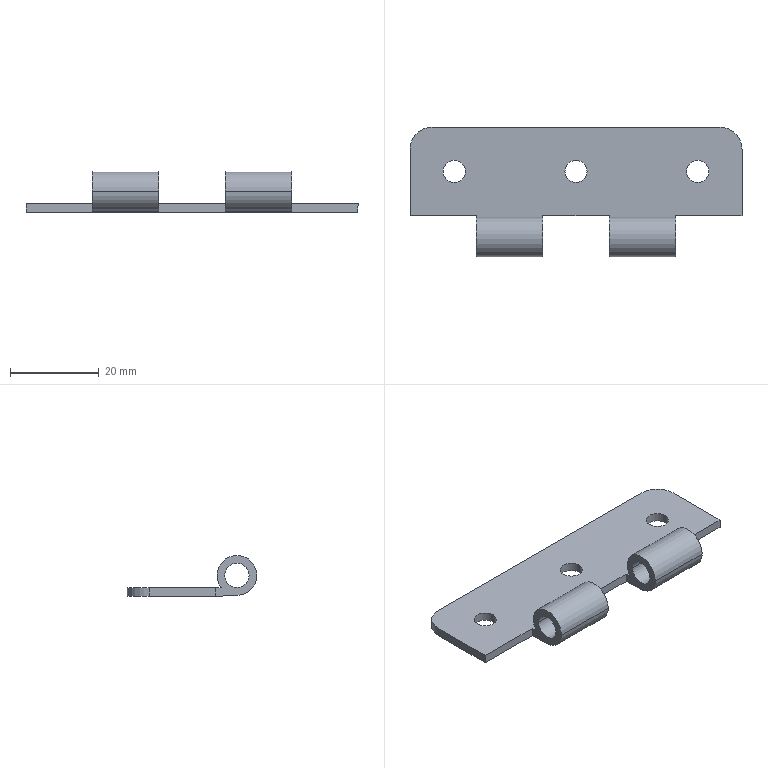Part | SolidWorks | features Extrusion 1, Fillet 1, ICE 1, LPattern 1 | 1 solid | 32 faces | box 75 x 29.3 x 9.25 mm | volume 4196 mm3 | cylinder 18 | plane 14 | commonest cylinder face diameters 5 x6 9 x6 5.5 x4 10 x2
STEP:
#1=CARTESIAN_POINT('',(60.,-22.05,4.75));
#2=VERTEX_POINT('',#1);
#3=CARTESIAN_POINT('',(60.,-27.55,4.75));
#4=VERTEX_POINT('',#3);
#5=CARTESIAN_POINT('',(60.,-24.8,4.75));
#6=DIRECTION('',(-1.,0.,0.));
#7=DIRECTION('',(0.,-1.,0.));
#8=AXIS2_PLACEMENT_3D('',#5,#6,#7);
#9=CIRCLE('',#8,2.75);
#10=EDGE_CURVE('',#2,#4,#9,.T.);
#11=ORIENTED_EDGE('',*,*,#10,.F.);
#12=CARTESIAN_POINT('',(45.,-22.05,4.75));
#13=VERTEX_POINT('',#12);
#14=CARTESIAN_POINT('',(60.,-22.05,4.75));
#15=DIRECTION('',(-1.,0.,0.));
#16=VECTOR('',#15,1000.);
#17=LINE('',#14,#16);
#18=EDGE_CURVE('',#2,#13,#17,.T.);
#19=ORIENTED_EDGE('',*,*,#18,.T.);
#20=CARTESIAN_POINT('',(45.,-27.55,4.75));
#21=VERTEX_POINT('',#20);
#22=CARTESIAN_POINT('',(45.,-24.8,4.75));
#23=DIRECTION('',(-1.,0.,0.));
#24=DIRECTION('',(0.,-1.,0.));
#25=AXIS2_PLACEMENT_3D('',#22,#23,#24);
#26=CIRCLE('',#25,2.75);
#27=EDGE_CURVE('',#13,#21,#26,.T.);
#28=ORIENTED_EDGE('',*,*,#27,.T.);
#29=CARTESIAN_POINT('',(60.,-27.55,4.75));
#30=DIRECTION('',(-1.,0.,0.));
#31=VECTOR('',#30,1000.);
#32=LINE('',#29,#31);
#33=EDGE_CURVE('',#4,#21,#32,.T.);
#34=ORIENTED_EDGE('',*,*,#33,.F.);
#35=EDGE_LOOP('',(#11,#19,#28,#34));
#36=FACE_OUTER_BOUND('',#35,.T.);
#37=CARTESIAN_POINT('',(60.,-24.8,4.75));
#38=DIRECTION('',(-1.,0.,0.));
#39=DIRECTION('',(0.,-1.,0.));
#40=AXIS2_PLACEMENT_3D('',#37,#38,#39);
#41=CYLINDRICAL_SURFACE('',#40,2.75);
#42=ADVANCED_FACE('',(#36),#41,.F.);
#43=CARTESIAN_POINT('',(60.,-29.3,4.75));
#44=VERTEX_POINT('',#43);
#45=CARTESIAN_POINT('',(60.,-20.3,4.75));
#46=VERTEX_POINT('',#45);
#47=CARTESIAN_POINT('',(60.,-24.8,4.75));
#48=DIRECTION('',(-1.,0.,0.));
#49=DIRECTION('',(0.,-1.,0.));
#50=AXIS2_PLACEMENT_3D('',#47,#48,#49);
#51=CIRCLE('',#50,4.5);
#52=EDGE_CURVE('',#44,#46,#51,.T.);
#53=ORIENTED_EDGE('',*,*,#52,.T.);
#54=CARTESIAN_POINT('',(45.,-20.3,4.75));
#55=VERTEX_POINT('',#54);
#56=CARTESIAN_POINT('',(60.,-20.3,4.75));
#57=DIRECTION('',(-1.,0.,0.));
#58=VECTOR('',#57,1000.);
#59=LINE('',#56,#58);
#60=EDGE_CURVE('',#46,#55,#59,.T.);
#61=ORIENTED_EDGE('',*,*,#60,.T.);
#62=CARTESIAN_POINT('',(45.,-29.3,4.75));
#63=VERTEX_POINT('',#62);
#64=CARTESIAN_POINT('',(45.,-24.8,4.75));
#65=DIRECTION('',(-1.,0.,0.));
#66=DIRECTION('',(0.,-1.,0.));
#67=AXIS2_PLACEMENT_3D('',#64,#65,#66);
#68=CIRCLE('',#67,4.5);
#69=EDGE_CURVE('',#63,#55,#68,.T.);
#70=ORIENTED_EDGE('',*,*,#69,.F.);
#71=CARTESIAN_POINT('',(60.,-29.3,4.75));
#72=DIRECTION('',(-1.,0.,0.));
#73=VECTOR('',#72,1000.);
#74=LINE('',#71,#73);
#75=EDGE_CURVE('',#44,#63,#74,.T.);
#76=ORIENTED_EDGE('',*,*,#75,.F.);
#77=EDGE_LOOP('',(#53,#61,#70,#76));
#78=FACE_OUTER_BOUND('',#77,.T.);
#79=CARTESIAN_POINT('',(60.,-24.8,4.75));
#80=DIRECTION('',(-1.,0.,0.));
#81=DIRECTION('',(0.,-1.,0.));
#82=AXIS2_PLACEMENT_3D('',#79,#80,#81);
#83=CYLINDRICAL_SURFACE('',#82,4.5);
#84=ADVANCED_FACE('',(#78),#83,.T.);
#85=CARTESIAN_POINT('',(60.,-25.029,0.2558));
#86=VERTEX_POINT('',#85);
#87=CARTESIAN_POINT('',(60.,-24.8,4.75));
#88=DIRECTION('',(-1.,0.,0.));
#89=DIRECTION('',(0.,-1.,0.));
#90=AXIS2_PLACEMENT_3D('',#87,#88,#89);
#91=CIRCLE('',#90,4.5);
#92=EDGE_CURVE('',#86,#44,#91,.T.);
#93=ORIENTED_EDGE('',*,*,#92,.T.);
#94=ORIENTED_EDGE('',*,*,#75,.T.);
#95=CARTESIAN_POINT('',(45.,-25.029,0.2558));
#96=VERTEX_POINT('',#95);
#97=CARTESIAN_POINT('',(45.,-24.8,4.75));
#98=DIRECTION('',(-1.,0.,0.));
#99=DIRECTION('',(0.,-1.,0.));
#100=AXIS2_PLACEMENT_3D('',#97,#98,#99);
#101=CIRCLE('',#100,4.5);
#102=EDGE_CURVE('',#96,#63,#101,.T.);
#103=ORIENTED_EDGE('',*,*,#102,.F.);
#104=CARTESIAN_POINT('',(60.,-25.029,0.2558));
#105=DIRECTION('',(-1.,0.,0.));
#106=VECTOR('',#105,1000.);
#107=LINE('',#104,#106);
#108=EDGE_CURVE('',#86,#96,#107,.T.);
#109=ORIENTED_EDGE('',*,*,#108,.F.);
#110=EDGE_LOOP('',(#93,#94,#103,#109));
#111=FACE_OUTER_BOUND('',#110,.T.);
#112=CARTESIAN_POINT('',(60.,-24.8,4.75));
#113=DIRECTION('',(-1.,0.,0.));
#114=DIRECTION('',(0.,-1.,0.));
#115=AXIS2_PLACEMENT_3D('',#112,#113,#114);
#116=CYLINDRICAL_SURFACE('',#115,4.5);
#117=ADVANCED_FACE('',(#111),#116,.T.);
#118=CARTESIAN_POINT('',(30.,-22.05,4.75));
#119=VERTEX_POINT('',#118);
#120=CARTESIAN_POINT('',(30.,-27.55,4.75));
#121=VERTEX_POINT('',#120);
#122=CARTESIAN_POINT('',(30.,-24.8,4.75));
#123=DIRECTION('',(-1.,0.,0.));
#124=DIRECTION('',(0.,-1.,0.));
#125=AXIS2_PLACEMENT_3D('',#122,#123,#124);
#126=CIRCLE('',#125,2.75);
#127=EDGE_CURVE('',#119,#121,#126,.T.);
#128=ORIENTED_EDGE('',*,*,#127,.F.);
#129=CARTESIAN_POINT('',(15.,-22.05,4.75));
#130=VERTEX_POINT('',#129);
#131=CARTESIAN_POINT('',(30.,-22.05,4.75));
#132=DIRECTION('',(-1.,0.,0.));
#133=VECTOR('',#132,1000.);
#134=LINE('',#131,#133);
#135=EDGE_CURVE('',#119,#130,#134,.T.);
#136=ORIENTED_EDGE('',*,*,#135,.T.);
#137=CARTESIAN_POINT('',(15.,-27.55,4.75));
#138=VERTEX_POINT('',#137);
#139=CARTESIAN_POINT('',(15.,-24.8,4.75));
#140=DIRECTION('',(-1.,0.,0.));
#141=DIRECTION('',(0.,-1.,0.));
#142=AXIS2_PLACEMENT_3D('',#139,#140,#141);
#143=CIRCLE('',#142,2.75);
#144=EDGE_CURVE('',#130,#138,#143,.T.);
#145=ORIENTED_EDGE('',*,*,#144,.T.);
#146=CARTESIAN_POINT('',(30.,-27.55,4.75));
#147=DIRECTION('',(-1.,0.,0.));
#148=VECTOR('',#147,1000.);
#149=LINE('',#146,#148);
#150=EDGE_CURVE('',#121,#138,#149,.T.);
#151=ORIENTED_EDGE('',*,*,#150,.F.);
#152=EDGE_LOOP('',(#128,#136,#145,#151));
#153=FACE_OUTER_BOUND('',#152,.T.);
#154=CARTESIAN_POINT('',(30.,-24.8,4.75));
#155=DIRECTION('',(-1.,0.,0.));
#156=DIRECTION('',(0.,-1.,0.));
#157=AXIS2_PLACEMENT_3D('',#154,#155,#156);
#158=CYLINDRICAL_SURFACE('',#157,2.75);
#159=ADVANCED_FACE('',(#153),#158,.F.);
#160=CARTESIAN_POINT('',(30.,-29.3,4.75));
#161=VERTEX_POINT('',#160);
#162=CARTESIAN_POINT('',(30.,-20.3,4.75));
#163=VERTEX_POINT('',#162);
#164=CARTESIAN_POINT('',(30.,-24.8,4.75));
#165=DIRECTION('',(-1.,0.,0.));
#166=DIRECTION('',(0.,-1.,0.));
#167=AXIS2_PLACEMENT_3D('',#164,#165,#166);
#168=CIRCLE('',#167,4.5);
#169=EDGE_CURVE('',#161,#163,#168,.T.);
#170=ORIENTED_EDGE('',*,*,#169,.T.);
#171=CARTESIAN_POINT('',(15.,-20.3,4.75));
#172=VERTEX_POINT('',#171);
#173=CARTESIAN_POINT('',(30.,-20.3,4.75));
#174=DIRECTION('',(-1.,0.,0.));
#175=VECTOR('',#174,1000.);
#176=LINE('',#173,#175);
#177=EDGE_CURVE('',#163,#172,#176,.T.);
#178=ORIENTED_EDGE('',*,*,#177,.T.);
#179=CARTESIAN_POINT('',(15.,-29.3,4.75));
#180=VERTEX_POINT('',#179);
#181=CARTESIAN_POINT('',(15.,-24.8,4.75));
#182=DIRECTION('',(-1.,0.,0.));
#183=DIRECTION('',(0.,-1.,0.));
#184=AXIS2_PLACEMENT_3D('',#181,#182,#183);
#185=CIRCLE('',#184,4.5);
#186=EDGE_CURVE('',#180,#172,#185,.T.);
#187=ORIENTED_EDGE('',*,*,#186,.F.);
#188=CARTESIAN_POINT('',(30.,-29.3,4.75));
#189=DIRECTION('',(-1.,0.,0.));
#190=VECTOR('',#189,1000.);
#191=LINE('',#188,#190);
#192=EDGE_CURVE('',#161,#180,#191,.T.);
#193=ORIENTED_EDGE('',*,*,#192,.F.);
#194=EDGE_LOOP('',(#170,#178,#187,#193));
#195=FACE_OUTER_BOUND('',#194,.T.);
#196=CARTESIAN_POINT('',(30.,-24.8,4.75));
#197=DIRECTION('',(-1.,0.,0.));
#198=DIRECTION('',(0.,-1.,0.));
#199=AXIS2_PLACEMENT_3D('',#196,#197,#198);
#200=CYLINDRICAL_SURFACE('',#199,4.5);
#201=ADVANCED_FACE('',(#195),#200,.T.);
#202=CARTESIAN_POINT('',(30.,-25.029,0.2558));
#203=VERTEX_POINT('',#202);
#204=CARTESIAN_POINT('',(30.,-24.8,4.75));
#205=DIRECTION('',(-1.,0.,0.));
#206=DIRECTION('',(0.,-1.,0.));
#207=AXIS2_PLACEMENT_3D('',#204,#205,#206);
#208=CIRCLE('',#207,4.5);
#209=EDGE_CURVE('',#203,#161,#208,.T.);
#210=ORIENTED_EDGE('',*,*,#209,.T.);
#211=ORIENTED_EDGE('',*,*,#192,.T.);
#212=CARTESIAN_POINT('',(15.,-25.029,0.2558));
#213=VERTEX_POINT('',#212);
#214=CARTESIAN_POINT('',(15.,-24.8,4.75));
#215=DIRECTION('',(-1.,0.,0.));
#216=DIRECTION('',(0.,-1.,0.));
#217=AXIS2_PLACEMENT_3D('',#214,#215,#216);
#218=CIRCLE('',#217,4.5);
#219=EDGE_CURVE('',#213,#180,#218,.T.);
#220=ORIENTED_EDGE('',*,*,#219,.F.);
#221=CARTESIAN_POINT('',(30.,-25.029,0.2558));
#222=DIRECTION('',(-1.,0.,0.));
#223=VECTOR('',#222,1000.);
#224=LINE('',#221,#223);
#225=EDGE_CURVE('',#203,#213,#224,.T.);
#226=ORIENTED_EDGE('',*,*,#225,.F.);
#227=EDGE_LOOP('',(#210,#211,#220,#226));
#228=FACE_OUTER_BOUND('',#227,.T.);
#229=CARTESIAN_POINT('',(30.,-24.8,4.75));
#230=DIRECTION('',(-1.,0.,0.));
#231=DIRECTION('',(0.,-1.,0.));
#232=AXIS2_PLACEMENT_3D('',#229,#230,#231);
#233=CYLINDRICAL_SURFACE('',#232,4.5);
#234=ADVANCED_FACE('',(#228),#233,.T.);
#235=CARTESIAN_POINT('',(35.,-10.,2.));
#236=VERTEX_POINT('',#235);
#237=CARTESIAN_POINT('',(40.,-10.,2.));
#238=VERTEX_POINT('',#237);
#239=CARTESIAN_POINT('',(37.5,-10.,2.));
#240=DIRECTION('',(0.,0.,1.));
#241=DIRECTION('',(1.,0.,0.));
#242=AXIS2_PLACEMENT_3D('',#239,#240,#241);
#243=CIRCLE('',#242,2.5);
#244=EDGE_CURVE('',#236,#238,#243,.T.);
#245=ORIENTED_EDGE('',*,*,#244,.T.);
#246=CARTESIAN_POINT('',(40.,-10.,0.));
#247=VERTEX_POINT('',#246);
#248=CARTESIAN_POINT('',(40.,-10.,2.));
#249=DIRECTION('',(0.,0.,-1.));
#250=VECTOR('',#249,1000.);
#251=LINE('',#248,#250);
#252=EDGE_CURVE('',#238,#247,#251,.T.);
#253=ORIENTED_EDGE('',*,*,#252,.T.);
#254=CARTESIAN_POINT('',(35.,-10.,0.));
#255=VERTEX_POINT('',#254);
#256=CARTESIAN_POINT('',(37.5,-10.,0.));
#257=DIRECTION('',(0.,0.,1.));
#258=DIRECTION('',(1.,0.,0.));
#259=AXIS2_PLACEMENT_3D('',#256,#257,#258);
#260=CIRCLE('',#259,2.5);
#261=EDGE_CURVE('',#255,#247,#260,.T.);
#262=ORIENTED_EDGE('',*,*,#261,.F.);
#263=CARTESIAN_POINT('',(35.,-10.,2.));
#264=DIRECTION('',(0.,0.,-1.));
#265=VECTOR('',#264,1000.);
#266=LINE('',#263,#265);
#267=EDGE_CURVE('',#236,#255,#266,.T.);
#268=ORIENTED_EDGE('',*,*,#267,.F.);
#269=EDGE_LOOP('',(#245,#253,#262,#268));
#270=FACE_OUTER_BOUND('',#269,.T.);
#271=CARTESIAN_POINT('',(37.5,-10.,2.));
#272=DIRECTION('',(0.,0.,-1.));
#273=DIRECTION('',(-1.,0.,0.));
#274=AXIS2_PLACEMENT_3D('',#271,#272,#273);
#275=CYLINDRICAL_SURFACE('',#274,2.5);
#276=ADVANCED_FACE('',(#270),#275,.F.);
#277=CARTESIAN_POINT('',(62.5,-10.,2.));
#278=VERTEX_POINT('',#277);
#279=CARTESIAN_POINT('',(67.5,-10.,2.));
#280=VERTEX_POINT('',#279);
#281=CARTESIAN_POINT('',(65.,-10.,2.));
#282=DIRECTION('',(0.,0.,1.));
#283=DIRECTION('',(1.,0.,0.));
#284=AXIS2_PLACEMENT_3D('',#281,#282,#283);
#285=CIRCLE('',#284,2.5);
#286=EDGE_CURVE('',#278,#280,#285,.T.);
#287=ORIENTED_EDGE('',*,*,#286,.T.);
#288=CARTESIAN_POINT('',(67.5,-10.,0.));
#289=VERTEX_POINT('',#288);
#290=CARTESIAN_POINT('',(67.5,-10.,2.));
#291=DIRECTION('',(0.,0.,-1.));
#292=VECTOR('',#291,1000.);
#293=LINE('',#290,#292);
#294=EDGE_CURVE('',#280,#289,#293,.T.);
#295=ORIENTED_EDGE('',*,*,#294,.T.);
#296=CARTESIAN_POINT('',(62.5,-10.,0.));
#297=VERTEX_POINT('',#296);
#298=CARTESIAN_POINT('',(65.,-10.,0.));
#299=DIRECTION('',(0.,0.,1.));
#300=DIRECTION('',(1.,0.,0.));
#301=AXIS2_PLACEMENT_3D('',#298,#299,#300);
#302=CIRCLE('',#301,2.5);
#303=EDGE_CURVE('',#297,#289,#302,.T.);
#304=ORIENTED_EDGE('',*,*,#303,.F.);
#305=CARTESIAN_POINT('',(62.5,-10.,2.));
#306=DIRECTION('',(0.,0.,-1.));
#307=VECTOR('',#306,1000.);
#308=LINE('',#305,#307);
#309=EDGE_CURVE('',#278,#297,#308,.T.);
#310=ORIENTED_EDGE('',*,*,#309,.F.);
#311=EDGE_LOOP('',(#287,#295,#304,#310));
#312=FACE_OUTER_BOUND('',#311,.T.);
#313=CARTESIAN_POINT('',(65.,-10.,2.));
#314=DIRECTION('',(0.,0.,-1.));
#315=DIRECTION('',(-1.,0.,0.));
#316=AXIS2_PLACEMENT_3D('',#313,#314,#315);
#317=CYLINDRICAL_SURFACE('',#316,2.5);
#318=ADVANCED_FACE('',(#312),#317,.F.);
#319=CARTESIAN_POINT('',(7.5,-10.,2.));
#320=VERTEX_POINT('',#319);
#321=CARTESIAN_POINT('',(12.5,-10.,2.));
#322=VERTEX_POINT('',#321);
#323=CARTESIAN_POINT('',(10.,-10.,2.));
#324=DIRECTION('',(0.,0.,1.));
#325=DIRECTION('',(1.,0.,0.));
#326=AXIS2_PLACEMENT_3D('',#323,#324,#325);
#327=CIRCLE('',#326,2.5);
#328=EDGE_CURVE('',#320,#322,#327,.T.);
#329=ORIENTED_EDGE('',*,*,#328,.T.);
#330=CARTESIAN_POINT('',(12.5,-10.,0.));
#331=VERTEX_POINT('',#330);
#332=CARTESIAN_POINT('',(12.5,-10.,2.));
#333=DIRECTION('',(0.,0.,-1.));
#334=VECTOR('',#333,1000.);
#335=LINE('',#332,#334);
#336=EDGE_CURVE('',#322,#331,#335,.T.);
#337=ORIENTED_EDGE('',*,*,#336,.T.);
#338=CARTESIAN_POINT('',(7.5,-10.,0.));
#339=VERTEX_POINT('',#338);
#340=CARTESIAN_POINT('',(10.,-10.,0.));
#341=DIRECTION('',(0.,0.,1.));
#342=DIRECTION('',(1.,0.,0.));
#343=AXIS2_PLACEMENT_3D('',#340,#341,#342);
#344=CIRCLE('',#343,2.5);
#345=EDGE_CURVE('',#339,#331,#344,.T.);
#346=ORIENTED_EDGE('',*,*,#345,.F.);
#347=CARTESIAN_POINT('',(7.5,-10.,2.));
#348=DIRECTION('',(0.,0.,-1.));
#349=VECTOR('',#348,1000.);
#350=LINE('',#347,#349);
#351=EDGE_CURVE('',#320,#339,#350,.T.);
#352=ORIENTED_EDGE('',*,*,#351,.F.);
#353=EDGE_LOOP('',(#329,#337,#346,#352));
#354=FACE_OUTER_BOUND('',#353,.T.);
#355=CARTESIAN_POINT('',(10.,-10.,2.));
#356=DIRECTION('',(0.,0.,-1.));
#357=DIRECTION('',(-1.,0.,0.));
#358=AXIS2_PLACEMENT_3D('',#355,#356,#357);
#359=CYLINDRICAL_SURFACE('',#358,2.5);
#360=ADVANCED_FACE('',(#354),#359,.F.);
#361=CARTESIAN_POINT('',(60.,-20.,0.));
#362=VERTEX_POINT('',#361);
#363=CARTESIAN_POINT('',(60.,-20.,2.));
#364=VERTEX_POINT('',#363);
#365=CARTESIAN_POINT('',(60.,-20.,0.));
#366=DIRECTION('',(0.,0.,1.));
#367=VECTOR('',#366,1000.);
#368=LINE('',#365,#367);
#369=EDGE_CURVE('',#362,#364,#368,.T.);
#370=ORIENTED_EDGE('',*,*,#369,.F.);
#371=CARTESIAN_POINT('',(75.,-20.,0.));
#372=VERTEX_POINT('',#371);
#373=CARTESIAN_POINT('',(0.,-20.,0.));
#374=DIRECTION('',(1.,0.,0.));
#375=VECTOR('',#374,1000.);
#376=LINE('',#373,#375);
#377=EDGE_CURVE('',#362,#372,#376,.T.);
#378=ORIENTED_EDGE('',*,*,#377,.T.);
#379=CARTESIAN_POINT('',(75.,-20.,2.));
#380=VERTEX_POINT('',#379);
#381=CARTESIAN_POINT('',(75.,-20.,2.));
#382=DIRECTION('',(0.,0.,-1.));
#383=VECTOR('',#382,1000.);
#384=LINE('',#381,#383);
#385=EDGE_CURVE('',#380,#372,#384,.T.);
#386=ORIENTED_EDGE('',*,*,#385,.F.);
#387=CARTESIAN_POINT('',(0.,-20.,2.));
#388=DIRECTION('',(1.,0.,0.));
#389=VECTOR('',#388,1000.);
#390=LINE('',#387,#389);
#391=EDGE_CURVE('',#364,#380,#390,.T.);
#392=ORIENTED_EDGE('',*,*,#391,.F.);
#393=EDGE_LOOP('',(#370,#378,#386,#392));
#394=FACE_OUTER_BOUND('',#393,.T.);
#395=CARTESIAN_POINT('',(0.,-20.,2.));
#396=DIRECTION('',(0.,1.,0.));
#397=DIRECTION('',(0.,0.,1.));
#398=AXIS2_PLACEMENT_3D('',#395,#396,#397);
#399=PLANE('',#398);
#400=ADVANCED_FACE('',(#394),#399,.F.);
#401=CARTESIAN_POINT('',(30.,-20.,0.));
#402=VERTEX_POINT('',#401);
#403=CARTESIAN_POINT('',(45.,-20.,0.));
#404=VERTEX_POINT('',#403);
#405=CARTESIAN_POINT('',(0.,-20.,0.));
#406=DIRECTION('',(1.,0.,0.));
#407=VECTOR('',#406,1000.);
#408=LINE('',#405,#407);
#409=EDGE_CURVE('',#402,#404,#408,.T.);
#410=ORIENTED_EDGE('',*,*,#409,.T.);
#411=CARTESIAN_POINT('',(45.,-20.,2.));
#412=VERTEX_POINT('',#411);
#413=CARTESIAN_POINT('',(45.,-20.,0.));
#414=DIRECTION('',(0.,0.,1.));
#415=VECTOR('',#414,1000.);
#416=LINE('',#413,#415);
#417=EDGE_CURVE('',#404,#412,#416,.T.);
#418=ORIENTED_EDGE('',*,*,#417,.T.);
#419=CARTESIAN_POINT('',(30.,-20.,2.));
#420=VERTEX_POINT('',#419);
#421=CARTESIAN_POINT('',(0.,-20.,2.));
#422=DIRECTION('',(1.,0.,0.));
#423=VECTOR('',#422,1000.);
#424=LINE('',#421,#423);
#425=EDGE_CURVE('',#420,#412,#424,.T.);
#426=ORIENTED_EDGE('',*,*,#425,.F.);
#427=CARTESIAN_POINT('',(30.,-20.,0.));
#428=DIRECTION('',(0.,0.,1.));
#429=VECTOR('',#428,1000.);
#430=LINE('',#427,#429);
#431=EDGE_CURVE('',#402,#420,#430,.T.);
#432=ORIENTED_EDGE('',*,*,#431,.F.);
#433=EDGE_LOOP('',(#410,#418,#426,#432));
#434=FACE_OUTER_BOUND('',#433,.T.);
#435=CARTESIAN_POINT('',(0.,-20.,2.));
#436=DIRECTION('',(0.,1.,0.));
#437=DIRECTION('',(0.,0.,1.));
#438=AXIS2_PLACEMENT_3D('',#435,#436,#437);
#439=PLANE('',#438);
#440=ADVANCED_FACE('',(#434),#439,.F.);
#441=ORIENTED_EDGE('',*,*,#286,.F.);
#442=CARTESIAN_POINT('',(65.,-10.,2.));
#443=DIRECTION('',(0.,0.,1.));
#444=DIRECTION('',(1.,0.,0.));
#445=AXIS2_PLACEMENT_3D('',#442,#443,#444);
#446=CIRCLE('',#445,2.5);
#447=EDGE_CURVE('',#280,#278,#446,.T.);
#448=ORIENTED_EDGE('',*,*,#447,.F.);
#449=EDGE_LOOP('',(#441,#448));
#450=FACE_BOUND('',#449,.T.);
#451=CARTESIAN_POINT('',(75.,-5.,2.));
#452=VERTEX_POINT('',#451);
#453=CARTESIAN_POINT('',(75.,0.,2.));
#454=DIRECTION('',(0.,1.,0.));
#455=VECTOR('',#454,1000.);
#456=LINE('',#453,#455);
#457=EDGE_CURVE('',#380,#452,#456,.T.);
#458=ORIENTED_EDGE('',*,*,#457,.T.);
#459=CARTESIAN_POINT('',(70.,0.,2.));
#460=VERTEX_POINT('',#459);
#461=CARTESIAN_POINT('',(70.,-5.,2.));
#462=DIRECTION('',(0.,0.,1.));
#463=DIRECTION('',(1.,0.,0.));
#464=AXIS2_PLACEMENT_3D('',#461,#462,#463);
#465=CIRCLE('',#464,5.);
#466=EDGE_CURVE('',#452,#460,#465,.T.);
#467=ORIENTED_EDGE('',*,*,#466,.T.);
#468=CARTESIAN_POINT('',(5.,0.,2.));
#469=VERTEX_POINT('',#468);
#470=CARTESIAN_POINT('',(0.,0.,2.));
#471=DIRECTION('',(-1.,0.,0.));
#472=VECTOR('',#471,1000.);
#473=LINE('',#470,#472);
#474=EDGE_CURVE('',#460,#469,#473,.T.);
#475=ORIENTED_EDGE('',*,*,#474,.T.);
#476=CARTESIAN_POINT('',(0.,-5.,2.));
#477=VERTEX_POINT('',#476);
#478=CARTESIAN_POINT('',(5.,-5.,2.));
#479=DIRECTION('',(0.,0.,1.));
#480=DIRECTION('',(1.,0.,0.));
#481=AXIS2_PLACEMENT_3D('',#478,#479,#480);
#482=CIRCLE('',#481,5.);
#483=EDGE_CURVE('',#469,#477,#482,.T.);
#484=ORIENTED_EDGE('',*,*,#483,.T.);
#485=CARTESIAN_POINT('',(0.,-20.,2.));
#486=VERTEX_POINT('',#485);
#487=CARTESIAN_POINT('',(0.,0.,2.));
#488=DIRECTION('',(0.,-1.,0.));
#489=VECTOR('',#488,1000.);
#490=LINE('',#487,#489);
#491=EDGE_CURVE('',#477,#486,#490,.T.);
#492=ORIENTED_EDGE('',*,*,#491,.T.);
#493=CARTESIAN_POINT('',(15.,-20.,2.));
#494=VERTEX_POINT('',#493);
#495=CARTESIAN_POINT('',(0.,-20.,2.));
#496=DIRECTION('',(1.,0.,0.));
#497=VECTOR('',#496,1000.);
#498=LINE('',#495,#497);
#499=EDGE_CURVE('',#486,#494,#498,.T.);
#500=ORIENTED_EDGE('',*,*,#499,.T.);
#501=CARTESIAN_POINT('',(15.,-21.238,2.));
#502=VERTEX_POINT('',#501);
#503=CARTESIAN_POINT('',(15.,0.,2.));
#504=DIRECTION('',(0.,-1.,0.));
#505=VECTOR('',#504,1000.);
#506=LINE('',#503,#505);
#507=EDGE_CURVE('',#494,#502,#506,.T.);
#508=ORIENTED_EDGE('',*,*,#507,.T.);
#509=CARTESIAN_POINT('',(30.,-21.238,2.));
#510=VERTEX_POINT('',#509);
#511=CARTESIAN_POINT('',(30.,-21.238,2.));
#512=DIRECTION('',(-1.,0.,0.));
#513=VECTOR('',#512,1000.);
#514=LINE('',#511,#513);
#515=EDGE_CURVE('',#510,#502,#514,.T.);
#516=ORIENTED_EDGE('',*,*,#515,.F.);
#517=CARTESIAN_POINT('',(30.,0.,2.));
#518=DIRECTION('',(0.,-1.,0.));
#519=VECTOR('',#518,1000.);
#520=LINE('',#517,#519);
#521=EDGE_CURVE('',#420,#510,#520,.T.);
#522=ORIENTED_EDGE('',*,*,#521,.F.);
#523=ORIENTED_EDGE('',*,*,#425,.T.);
#524=CARTESIAN_POINT('',(45.,-21.238,2.));
#525=VERTEX_POINT('',#524);
#526=CARTESIAN_POINT('',(45.,0.,2.));
#527=DIRECTION('',(0.,-1.,0.));
#528=VECTOR('',#527,1000.);
#529=LINE('',#526,#528);
#530=EDGE_CURVE('',#412,#525,#529,.T.);
#531=ORIENTED_EDGE('',*,*,#530,.T.);
#532=CARTESIAN_POINT('',(60.,-21.238,2.));
#533=VERTEX_POINT('',#532);
#534=CARTESIAN_POINT('',(60.,-21.238,2.));
#535=DIRECTION('',(-1.,0.,0.));
#536=VECTOR('',#535,1000.);
#537=LINE('',#534,#536);
#538=EDGE_CURVE('',#533,#525,#537,.T.);
#539=ORIENTED_EDGE('',*,*,#538,.F.);
#540=CARTESIAN_POINT('',(60.,0.,2.));
#541=DIRECTION('',(0.,-1.,0.));
#542=VECTOR('',#541,1000.);
#543=LINE('',#540,#542);
#544=EDGE_CURVE('',#364,#533,#543,.T.);
#545=ORIENTED_EDGE('',*,*,#544,.F.);
#546=ORIENTED_EDGE('',*,*,#391,.T.);
#547=EDGE_LOOP('',(#458,#467,#475,#484,#492,#500,#508,#516,#522,#523,#531,#539,#545,#546));
#548=FACE_OUTER_BOUND('',#547,.T.);
#549=ORIENTED_EDGE('',*,*,#328,.F.);
#550=CARTESIAN_POINT('',(10.,-10.,2.));
#551=DIRECTION('',(0.,0.,1.));
#552=DIRECTION('',(1.,0.,0.));
#553=AXIS2_PLACEMENT_3D('',#550,#551,#552);
#554=CIRCLE('',#553,2.5);
#555=EDGE_CURVE('',#322,#320,#554,.T.);
#556=ORIENTED_EDGE('',*,*,#555,.F.);
#557=EDGE_LOOP('',(#549,#556));
#558=FACE_BOUND('',#557,.T.);
#559=ORIENTED_EDGE('',*,*,#244,.F.);
#560=CARTESIAN_POINT('',(37.5,-10.,2.));
#561=DIRECTION('',(0.,0.,1.));
#562=DIRECTION('',(1.,0.,0.));
#563=AXIS2_PLACEMENT_3D('',#560,#561,#562);
#564=CIRCLE('',#563,2.5);
#565=EDGE_CURVE('',#238,#236,#564,.T.);
#566=ORIENTED_EDGE('',*,*,#565,.F.);
#567=EDGE_LOOP('',(#559,#566));
#568=FACE_BOUND('',#567,.T.);
#569=CARTESIAN_POINT('',(0.,0.,2.));
#570=DIRECTION('',(0.,0.,1.));
#571=DIRECTION('',(1.,0.,0.));
#572=AXIS2_PLACEMENT_3D('',#569,#570,#571);
#573=PLANE('',#572);
#574=ADVANCED_FACE('',(#450,#548,#558,#568),#573,.T.);
#575=CARTESIAN_POINT('',(70.,0.,0.));
#576=VERTEX_POINT('',#575);
#577=CARTESIAN_POINT('',(5.,0.,0.));
#578=VERTEX_POINT('',#577);
#579=CARTESIAN_POINT('',(0.,0.,0.));
#580=DIRECTION('',(-1.,0.,0.));
#581=VECTOR('',#580,1000.);
#582=LINE('',#579,#581);
#583=EDGE_CURVE('',#576,#578,#582,.T.);
#584=ORIENTED_EDGE('',*,*,#583,.F.);
#585=CARTESIAN_POINT('',(75.,-5.,0.));
#586=VERTEX_POINT('',#585);
#587=CARTESIAN_POINT('',(70.,-5.,0.));
#588=DIRECTION('',(0.,0.,-1.));
#589=DIRECTION('',(1.,0.,0.));
#590=AXIS2_PLACEMENT_3D('',#587,#588,#589);
#591=CIRCLE('',#590,5.);
#592=EDGE_CURVE('',#576,#586,#591,.T.);
#593=ORIENTED_EDGE('',*,*,#592,.T.);
#594=CARTESIAN_POINT('',(75.,0.,0.));
#595=DIRECTION('',(0.,1.,0.));
#596=VECTOR('',#595,1000.);
#597=LINE('',#594,#596);
#598=EDGE_CURVE('',#372,#586,#597,.T.);
#599=ORIENTED_EDGE('',*,*,#598,.F.);
#600=ORIENTED_EDGE('',*,*,#377,.F.);
#601=CARTESIAN_POINT('',(60.,-20.,0.));
#602=DIRECTION('',(-1.,0.,0.));
#603=VECTOR('',#602,1000.);
#604=LINE('',#601,#603);
#605=EDGE_CURVE('',#362,#404,#604,.T.);
#606=ORIENTED_EDGE('',*,*,#605,.T.);
#607=ORIENTED_EDGE('',*,*,#409,.F.);
#608=CARTESIAN_POINT('',(15.,-20.,0.));
#609=VERTEX_POINT('',#608);
#610=CARTESIAN_POINT('',(30.,-20.,0.));
#611=DIRECTION('',(-1.,0.,0.));
#612=VECTOR('',#611,1000.);
#613=LINE('',#610,#612);
#614=EDGE_CURVE('',#402,#609,#613,.T.);
#615=ORIENTED_EDGE('',*,*,#614,.T.);
#616=CARTESIAN_POINT('',(0.,-20.,0.));
#617=VERTEX_POINT('',#616);
#618=CARTESIAN_POINT('',(0.,-20.,0.));
#619=DIRECTION('',(1.,0.,0.));
#620=VECTOR('',#619,1000.);
#621=LINE('',#618,#620);
#622=EDGE_CURVE('',#617,#609,#621,.T.);
#623=ORIENTED_EDGE('',*,*,#622,.F.);
#624=CARTESIAN_POINT('',(0.,-5.,0.));
#625=VERTEX_POINT('',#624);
#626=CARTESIAN_POINT('',(0.,0.,0.));
#627=DIRECTION('',(0.,-1.,0.));
#628=VECTOR('',#627,1000.);
#629=LINE('',#626,#628);
#630=EDGE_CURVE('',#625,#617,#629,.T.);
#631=ORIENTED_EDGE('',*,*,#630,.F.);
#632=CARTESIAN_POINT('',(5.,-5.,0.));
#633=DIRECTION('',(0.,0.,-1.));
#634=DIRECTION('',(1.,0.,0.));
#635=AXIS2_PLACEMENT_3D('',#632,#633,#634);
#636=CIRCLE('',#635,5.);
#637=EDGE_CURVE('',#625,#578,#636,.T.);
#638=ORIENTED_EDGE('',*,*,#637,.T.);
#639=EDGE_LOOP('',(#584,#593,#599,#600,#606,#607,#615,#623,#631,#638));
#640=FACE_OUTER_BOUND('',#639,.T.);
#641=ORIENTED_EDGE('',*,*,#345,.T.);
#642=CARTESIAN_POINT('',(10.,-10.,0.));
#643=DIRECTION('',(0.,0.,1.));
#644=DIRECTION('',(1.,0.,0.));
#645=AXIS2_PLACEMENT_3D('',#642,#643,#644);
#646=CIRCLE('',#645,2.5);
#647=EDGE_CURVE('',#331,#339,#646,.T.);
#648=ORIENTED_EDGE('',*,*,#647,.T.);
#649=EDGE_LOOP('',(#641,#648));
#650=FACE_BOUND('',#649,.T.);
#651=ORIENTED_EDGE('',*,*,#303,.T.);
#652=CARTESIAN_POINT('',(65.,-10.,0.));
#653=DIRECTION('',(0.,0.,1.));
#654=DIRECTION('',(1.,0.,0.));
#655=AXIS2_PLACEMENT_3D('',#652,#653,#654);
#656=CIRCLE('',#655,2.5);
#657=EDGE_CURVE('',#289,#297,#656,.T.);
#658=ORIENTED_EDGE('',*,*,#657,.T.);
#659=EDGE_LOOP('',(#651,#658));
#660=FACE_BOUND('',#659,.T.);
#661=ORIENTED_EDGE('',*,*,#261,.T.);
#662=CARTESIAN_POINT('',(37.5,-10.,0.));
#663=DIRECTION('',(0.,0.,1.));
#664=DIRECTION('',(1.,0.,0.));
#665=AXIS2_PLACEMENT_3D('',#662,#663,#664);
#666=CIRCLE('',#665,2.5);
#667=EDGE_CURVE('',#247,#255,#666,.T.);
#668=ORIENTED_EDGE('',*,*,#667,.T.);
#669=EDGE_LOOP('',(#661,#668));
#670=FACE_BOUND('',#669,.T.);
#671=CARTESIAN_POINT('',(0.,0.,0.));
#672=DIRECTION('',(0.,0.,1.));
#673=DIRECTION('',(1.,0.,0.));
#674=AXIS2_PLACEMENT_3D('',#671,#672,#673);
#675=PLANE('',#674);
#676=ADVANCED_FACE('',(#640,#650,#660,#670),#675,.F.);
#677=ORIENTED_EDGE('',*,*,#491,.F.);
#678=CARTESIAN_POINT('',(0.,-5.,2.));
#679=DIRECTION('',(0.,0.,-1.));
#680=VECTOR('',#679,1000.);
#681=LINE('',#678,#680);
#682=EDGE_CURVE('',#477,#625,#681,.T.);
#683=ORIENTED_EDGE('',*,*,#682,.T.);
#684=ORIENTED_EDGE('',*,*,#630,.T.);
#685=CARTESIAN_POINT('',(0.,-20.,2.));
#686=DIRECTION('',(0.,0.,-1.));
#687=VECTOR('',#686,1000.);
#688=LINE('',#685,#687);
#689=EDGE_CURVE('',#486,#617,#688,.T.);
#690=ORIENTED_EDGE('',*,*,#689,.F.);
#691=EDGE_LOOP('',(#677,#683,#684,#690));
#692=FACE_OUTER_BOUND('',#691,.T.);
#693=CARTESIAN_POINT('',(0.,0.,2.));
#694=DIRECTION('',(1.,0.,0.));
#695=DIRECTION('',(0.,1.,0.));
#696=AXIS2_PLACEMENT_3D('',#693,#694,#695);
#697=PLANE('',#696);
#698=ADVANCED_FACE('',(#692),#697,.F.);
#699=ORIENTED_EDGE('',*,*,#622,.T.);
#700=CARTESIAN_POINT('',(15.,-20.,0.));
#701=DIRECTION('',(0.,0.,1.));
#702=VECTOR('',#701,1000.);
#703=LINE('',#700,#702);
#704=EDGE_CURVE('',#609,#494,#703,.T.);
#705=ORIENTED_EDGE('',*,*,#704,.T.);
#706=ORIENTED_EDGE('',*,*,#499,.F.);
#707=ORIENTED_EDGE('',*,*,#689,.T.);
#708=EDGE_LOOP('',(#699,#705,#706,#707));
#709=FACE_OUTER_BOUND('',#708,.T.);
#710=CARTESIAN_POINT('',(0.,-20.,2.));
#711=DIRECTION('',(0.,1.,0.));
#712=DIRECTION('',(0.,0.,1.));
#713=AXIS2_PLACEMENT_3D('',#710,#711,#712);
#714=PLANE('',#713);
#715=ADVANCED_FACE('',(#709),#714,.F.);
#716=ORIENTED_EDGE('',*,*,#598,.T.);
#717=CARTESIAN_POINT('',(75.,-5.,2.));
#718=DIRECTION('',(0.,0.,1.));
#719=VECTOR('',#718,1000.);
#720=LINE('',#717,#719);
#721=EDGE_CURVE('',#586,#452,#720,.T.);
#722=ORIENTED_EDGE('',*,*,#721,.T.);
#723=ORIENTED_EDGE('',*,*,#457,.F.);
#724=ORIENTED_EDGE('',*,*,#385,.T.);
#725=EDGE_LOOP('',(#716,#722,#723,#724));
#726=FACE_OUTER_BOUND('',#725,.T.);
#727=CARTESIAN_POINT('',(75.,0.,2.));
#728=DIRECTION('',(-1.,0.,0.));
#729=DIRECTION('',(0.,0.,1.));
#730=AXIS2_PLACEMENT_3D('',#727,#728,#729);
#731=PLANE('',#730);
#732=ADVANCED_FACE('',(#726),#731,.F.);
#733=ORIENTED_EDGE('',*,*,#474,.F.);
#734=CARTESIAN_POINT('',(70.,0.,2.));
#735=DIRECTION('',(0.,0.,-1.));
#736=VECTOR('',#735,1000.);
#737=LINE('',#734,#736);
#738=EDGE_CURVE('',#460,#576,#737,.T.);
#739=ORIENTED_EDGE('',*,*,#738,.T.);
#740=ORIENTED_EDGE('',*,*,#583,.T.);
#741=CARTESIAN_POINT('',(5.,0.,2.));
#742=DIRECTION('',(0.,0.,1.));
#743=VECTOR('',#742,1000.);
#744=LINE('',#741,#743);
#745=EDGE_CURVE('',#578,#469,#744,.T.);
#746=ORIENTED_EDGE('',*,*,#745,.T.);
#747=EDGE_LOOP('',(#733,#739,#740,#746));
#748=FACE_OUTER_BOUND('',#747,.T.);
#749=CARTESIAN_POINT('',(0.,0.,2.));
#750=DIRECTION('',(0.,-1.,0.));
#751=DIRECTION('',(0.,0.,-1.));
#752=AXIS2_PLACEMENT_3D('',#749,#750,#751);
#753=PLANE('',#752);
#754=ADVANCED_FACE('',(#748),#753,.F.);
#755=ORIENTED_EDGE('',*,*,#336,.F.);
#756=ORIENTED_EDGE('',*,*,#555,.T.);
#757=ORIENTED_EDGE('',*,*,#351,.T.);
#758=ORIENTED_EDGE('',*,*,#647,.F.);
#759=EDGE_LOOP('',(#755,#756,#757,#758));
#760=FACE_OUTER_BOUND('',#759,.T.);
#761=CARTESIAN_POINT('',(10.,-10.,2.));
#762=DIRECTION('',(0.,0.,-1.));
#763=DIRECTION('',(-1.,0.,0.));
#764=AXIS2_PLACEMENT_3D('',#761,#762,#763);
#765=CYLINDRICAL_SURFACE('',#764,2.5);
#766=ADVANCED_FACE('',(#760),#765,.F.);
#767=ORIENTED_EDGE('',*,*,#294,.F.);
#768=ORIENTED_EDGE('',*,*,#447,.T.);
#769=ORIENTED_EDGE('',*,*,#309,.T.);
#770=ORIENTED_EDGE('',*,*,#657,.F.);
#771=EDGE_LOOP('',(#767,#768,#769,#770));
#772=FACE_OUTER_BOUND('',#771,.T.);
#773=CARTESIAN_POINT('',(65.,-10.,2.));
#774=DIRECTION('',(0.,0.,-1.));
#775=DIRECTION('',(-1.,0.,0.));
#776=AXIS2_PLACEMENT_3D('',#773,#774,#775);
#777=CYLINDRICAL_SURFACE('',#776,2.5);
#778=ADVANCED_FACE('',(#772),#777,.F.);
#779=ORIENTED_EDGE('',*,*,#252,.F.);
#780=ORIENTED_EDGE('',*,*,#565,.T.);
#781=ORIENTED_EDGE('',*,*,#267,.T.);
#782=ORIENTED_EDGE('',*,*,#667,.F.);
#783=EDGE_LOOP('',(#779,#780,#781,#782));
#784=FACE_OUTER_BOUND('',#783,.T.);
#785=CARTESIAN_POINT('',(37.5,-10.,2.));
#786=DIRECTION('',(0.,0.,-1.));
#787=DIRECTION('',(-1.,0.,0.));
#788=AXIS2_PLACEMENT_3D('',#785,#786,#787);
#789=CYLINDRICAL_SURFACE('',#788,2.5);
#790=ADVANCED_FACE('',(#784),#789,.F.);
#791=ORIENTED_EDGE('',*,*,#177,.F.);
#792=CARTESIAN_POINT('',(30.,-24.8,4.75));
#793=DIRECTION('',(-1.,0.,0.));
#794=DIRECTION('',(0.,-1.,0.));
#795=AXIS2_PLACEMENT_3D('',#792,#793,#794);
#796=CIRCLE('',#795,4.5);
#797=EDGE_CURVE('',#163,#510,#796,.T.);
#798=ORIENTED_EDGE('',*,*,#797,.T.);
#799=ORIENTED_EDGE('',*,*,#515,.T.);
#800=CARTESIAN_POINT('',(15.,-24.8,4.75));
#801=DIRECTION('',(-1.,0.,0.));
#802=DIRECTION('',(0.,-1.,0.));
#803=AXIS2_PLACEMENT_3D('',#800,#801,#802);
#804=CIRCLE('',#803,4.5);
#805=EDGE_CURVE('',#172,#502,#804,.T.);
#806=ORIENTED_EDGE('',*,*,#805,.F.);
#807=EDGE_LOOP('',(#791,#798,#799,#806));
#808=FACE_OUTER_BOUND('',#807,.T.);
#809=CARTESIAN_POINT('',(30.,-24.8,4.75));
#810=DIRECTION('',(-1.,0.,0.));
#811=DIRECTION('',(0.,-1.,0.));
#812=AXIS2_PLACEMENT_3D('',#809,#810,#811);
#813=CYLINDRICAL_SURFACE('',#812,4.5);
#814=ADVANCED_FACE('',(#808),#813,.T.);
#815=CARTESIAN_POINT('',(15.,-0.05162,-1.015));
#816=DIRECTION('',(0.,-0.9987,0.05081));
#817=VECTOR('',#816,1000.);
#818=LINE('',#815,#817);
#819=EDGE_CURVE('',#609,#213,#818,.T.);
#820=ORIENTED_EDGE('',*,*,#819,.F.);
#821=ORIENTED_EDGE('',*,*,#614,.F.);
#822=CARTESIAN_POINT('',(30.,-0.05162,-1.015));
#823=DIRECTION('',(0.,-0.9987,0.05081));
#824=VECTOR('',#823,1000.);
#825=LINE('',#822,#824);
#826=EDGE_CURVE('',#402,#203,#825,.T.);
#827=ORIENTED_EDGE('',*,*,#826,.T.);
#828=ORIENTED_EDGE('',*,*,#225,.T.);
#829=EDGE_LOOP('',(#820,#821,#827,#828));
#830=FACE_OUTER_BOUND('',#829,.T.);
#831=CARTESIAN_POINT('',(30.,-0.05162,-1.015));
#832=DIRECTION('',(0.,-0.05081,-0.9987));
#833=DIRECTION('',(0.,0.9987,-0.05081));
#834=AXIS2_PLACEMENT_3D('',#831,#832,#833);
#835=PLANE('',#834);
#836=ADVANCED_FACE('',(#830),#835,.T.);
#837=ORIENTED_EDGE('',*,*,#135,.F.);
#838=CARTESIAN_POINT('',(30.,-24.8,4.75));
#839=DIRECTION('',(-1.,0.,0.));
#840=DIRECTION('',(0.,-1.,0.));
#841=AXIS2_PLACEMENT_3D('',#838,#839,#840);
#842=CIRCLE('',#841,2.75);
#843=EDGE_CURVE('',#121,#119,#842,.T.);
#844=ORIENTED_EDGE('',*,*,#843,.F.);
#845=ORIENTED_EDGE('',*,*,#150,.T.);
#846=CARTESIAN_POINT('',(15.,-24.8,4.75));
#847=DIRECTION('',(-1.,0.,0.));
#848=DIRECTION('',(0.,-1.,0.));
#849=AXIS2_PLACEMENT_3D('',#846,#847,#848);
#850=CIRCLE('',#849,2.75);
#851=EDGE_CURVE('',#138,#130,#850,.T.);
#852=ORIENTED_EDGE('',*,*,#851,.T.);
#853=EDGE_LOOP('',(#837,#844,#845,#852));
#854=FACE_OUTER_BOUND('',#853,.T.);
#855=CARTESIAN_POINT('',(30.,-24.8,4.75));
#856=DIRECTION('',(-1.,0.,0.));
#857=DIRECTION('',(0.,-1.,0.));
#858=AXIS2_PLACEMENT_3D('',#855,#856,#857);
#859=CYLINDRICAL_SURFACE('',#858,2.75);
#860=ADVANCED_FACE('',(#854),#859,.F.);
#861=ORIENTED_EDGE('',*,*,#843,.T.);
#862=ORIENTED_EDGE('',*,*,#127,.T.);
#863=EDGE_LOOP('',(#861,#862));
#864=FACE_BOUND('',#863,.T.);
#865=ORIENTED_EDGE('',*,*,#209,.F.);
#866=ORIENTED_EDGE('',*,*,#826,.F.);
#867=ORIENTED_EDGE('',*,*,#431,.T.);
#868=ORIENTED_EDGE('',*,*,#521,.T.);
#869=ORIENTED_EDGE('',*,*,#797,.F.);
#870=ORIENTED_EDGE('',*,*,#169,.F.);
#871=EDGE_LOOP('',(#865,#866,#867,#868,#869,#870));
#872=FACE_OUTER_BOUND('',#871,.T.);
#873=CARTESIAN_POINT('',(30.,0.,0.));
#874=DIRECTION('',(-1.,0.,0.));
#875=DIRECTION('',(0.,-1.,0.));
#876=AXIS2_PLACEMENT_3D('',#873,#874,#875);
#877=PLANE('',#876);
#878=ADVANCED_FACE('',(#864,#872),#877,.F.);
#879=ORIENTED_EDGE('',*,*,#851,.F.);
#880=ORIENTED_EDGE('',*,*,#144,.F.);
#881=EDGE_LOOP('',(#879,#880));
#882=FACE_BOUND('',#881,.T.);
#883=ORIENTED_EDGE('',*,*,#219,.T.);
#884=ORIENTED_EDGE('',*,*,#186,.T.);
#885=ORIENTED_EDGE('',*,*,#805,.T.);
#886=ORIENTED_EDGE('',*,*,#507,.F.);
#887=ORIENTED_EDGE('',*,*,#704,.F.);
#888=ORIENTED_EDGE('',*,*,#819,.T.);
#889=EDGE_LOOP('',(#883,#884,#885,#886,#887,#888));
#890=FACE_OUTER_BOUND('',#889,.T.);
#891=CARTESIAN_POINT('',(15.,0.,0.));
#892=DIRECTION('',(-1.,0.,0.));
#893=DIRECTION('',(0.,-1.,0.));
#894=AXIS2_PLACEMENT_3D('',#891,#892,#893);
#895=PLANE('',#894);
#896=ADVANCED_FACE('',(#882,#890),#895,.T.);
#897=ORIENTED_EDGE('',*,*,#60,.F.);
#898=CARTESIAN_POINT('',(60.,-24.8,4.75));
#899=DIRECTION('',(-1.,0.,0.));
#900=DIRECTION('',(0.,-1.,0.));
#901=AXIS2_PLACEMENT_3D('',#898,#899,#900);
#902=CIRCLE('',#901,4.5);
#903=EDGE_CURVE('',#46,#533,#902,.T.);
#904=ORIENTED_EDGE('',*,*,#903,.T.);
#905=ORIENTED_EDGE('',*,*,#538,.T.);
#906=CARTESIAN_POINT('',(45.,-24.8,4.75));
#907=DIRECTION('',(-1.,0.,0.));
#908=DIRECTION('',(0.,-1.,0.));
#909=AXIS2_PLACEMENT_3D('',#906,#907,#908);
#910=CIRCLE('',#909,4.5);
#911=EDGE_CURVE('',#55,#525,#910,.T.);
#912=ORIENTED_EDGE('',*,*,#911,.F.);
#913=EDGE_LOOP('',(#897,#904,#905,#912));
#914=FACE_OUTER_BOUND('',#913,.T.);
#915=CARTESIAN_POINT('',(60.,-24.8,4.75));
#916=DIRECTION('',(-1.,0.,0.));
#917=DIRECTION('',(0.,-1.,0.));
#918=AXIS2_PLACEMENT_3D('',#915,#916,#917);
#919=CYLINDRICAL_SURFACE('',#918,4.5);
#920=ADVANCED_FACE('',(#914),#919,.T.);
#921=CARTESIAN_POINT('',(45.,-0.05162,-1.015));
#922=DIRECTION('',(0.,-0.9987,0.05081));
#923=VECTOR('',#922,1000.);
#924=LINE('',#921,#923);
#925=EDGE_CURVE('',#404,#96,#924,.T.);
#926=ORIENTED_EDGE('',*,*,#925,.F.);
#927=ORIENTED_EDGE('',*,*,#605,.F.);
#928=CARTESIAN_POINT('',(60.,-0.05162,-1.015));
#929=DIRECTION('',(0.,-0.9987,0.05081));
#930=VECTOR('',#929,1000.);
#931=LINE('',#928,#930);
#932=EDGE_CURVE('',#362,#86,#931,.T.);
#933=ORIENTED_EDGE('',*,*,#932,.T.);
#934=ORIENTED_EDGE('',*,*,#108,.T.);
#935=EDGE_LOOP('',(#926,#927,#933,#934));
#936=FACE_OUTER_BOUND('',#935,.T.);
#937=CARTESIAN_POINT('',(60.,-0.05162,-1.015));
#938=DIRECTION('',(0.,-0.05081,-0.9987));
#939=DIRECTION('',(0.,0.9987,-0.05081));
#940=AXIS2_PLACEMENT_3D('',#937,#938,#939);
#941=PLANE('',#940);
#942=ADVANCED_FACE('',(#936),#941,.T.);
#943=ORIENTED_EDGE('',*,*,#18,.F.);
#944=CARTESIAN_POINT('',(60.,-24.8,4.75));
#945=DIRECTION('',(-1.,0.,0.));
#946=DIRECTION('',(0.,-1.,0.));
#947=AXIS2_PLACEMENT_3D('',#944,#945,#946);
#948=CIRCLE('',#947,2.75);
#949=EDGE_CURVE('',#4,#2,#948,.T.);
#950=ORIENTED_EDGE('',*,*,#949,.F.);
#951=ORIENTED_EDGE('',*,*,#33,.T.);
#952=CARTESIAN_POINT('',(45.,-24.8,4.75));
#953=DIRECTION('',(-1.,0.,0.));
#954=DIRECTION('',(0.,-1.,0.));
#955=AXIS2_PLACEMENT_3D('',#952,#953,#954);
#956=CIRCLE('',#955,2.75);
#957=EDGE_CURVE('',#21,#13,#956,.T.);
#958=ORIENTED_EDGE('',*,*,#957,.T.);
#959=EDGE_LOOP('',(#943,#950,#951,#958));
#960=FACE_OUTER_BOUND('',#959,.T.);
#961=CARTESIAN_POINT('',(60.,-24.8,4.75));
#962=DIRECTION('',(-1.,0.,0.));
#963=DIRECTION('',(0.,-1.,0.));
#964=AXIS2_PLACEMENT_3D('',#961,#962,#963);
#965=CYLINDRICAL_SURFACE('',#964,2.75);
#966=ADVANCED_FACE('',(#960),#965,.F.);
#967=ORIENTED_EDGE('',*,*,#949,.T.);
#968=ORIENTED_EDGE('',*,*,#10,.T.);
#969=EDGE_LOOP('',(#967,#968));
#970=FACE_BOUND('',#969,.T.);
#971=ORIENTED_EDGE('',*,*,#92,.F.);
#972=ORIENTED_EDGE('',*,*,#932,.F.);
#973=ORIENTED_EDGE('',*,*,#369,.T.);
#974=ORIENTED_EDGE('',*,*,#544,.T.);
#975=ORIENTED_EDGE('',*,*,#903,.F.);
#976=ORIENTED_EDGE('',*,*,#52,.F.);
#977=EDGE_LOOP('',(#971,#972,#973,#974,#975,#976));
#978=FACE_OUTER_BOUND('',#977,.T.);
#979=CARTESIAN_POINT('',(60.,0.,0.));
#980=DIRECTION('',(-1.,0.,0.));
#981=DIRECTION('',(0.,-1.,0.));
#982=AXIS2_PLACEMENT_3D('',#979,#980,#981);
#983=PLANE('',#982);
#984=ADVANCED_FACE('',(#970,#978),#983,.F.);
#985=ORIENTED_EDGE('',*,*,#957,.F.);
#986=ORIENTED_EDGE('',*,*,#27,.F.);
#987=EDGE_LOOP('',(#985,#986));
#988=FACE_BOUND('',#987,.T.);
#989=ORIENTED_EDGE('',*,*,#102,.T.);
#990=ORIENTED_EDGE('',*,*,#69,.T.);
#991=ORIENTED_EDGE('',*,*,#911,.T.);
#992=ORIENTED_EDGE('',*,*,#530,.F.);
#993=ORIENTED_EDGE('',*,*,#417,.F.);
#994=ORIENTED_EDGE('',*,*,#925,.T.);
#995=EDGE_LOOP('',(#989,#990,#991,#992,#993,#994));
#996=FACE_OUTER_BOUND('',#995,.T.);
#997=CARTESIAN_POINT('',(45.,0.,0.));
#998=DIRECTION('',(-1.,0.,0.));
#999=DIRECTION('',(0.,-1.,0.));
#1000=AXIS2_PLACEMENT_3D('',#997,#998,#999);
#1001=PLANE('',#1000);
#1002=ADVANCED_FACE('',(#988,#996),#1001,.T.);
#1003=ORIENTED_EDGE('',*,*,#466,.F.);
#1004=ORIENTED_EDGE('',*,*,#721,.F.);
#1005=ORIENTED_EDGE('',*,*,#592,.F.);
#1006=ORIENTED_EDGE('',*,*,#738,.F.);
#1007=EDGE_LOOP('',(#1003,#1004,#1005,#1006));
#1008=FACE_OUTER_BOUND('',#1007,.T.);
#1009=CARTESIAN_POINT('',(70.,-5.,2.));
#1010=DIRECTION('',(0.,0.,-1.));
#1011=DIRECTION('',(-1.,0.,0.));
#1012=AXIS2_PLACEMENT_3D('',#1009,#1010,#1011);
#1013=CYLINDRICAL_SURFACE('',#1012,5.);
#1014=ADVANCED_FACE('',(#1008),#1013,.T.);
#1015=ORIENTED_EDGE('',*,*,#483,.F.);
#1016=ORIENTED_EDGE('',*,*,#745,.F.);
#1017=ORIENTED_EDGE('',*,*,#637,.F.);
#1018=ORIENTED_EDGE('',*,*,#682,.F.);
#1019=EDGE_LOOP('',(#1015,#1016,#1017,#1018));
#1020=FACE_OUTER_BOUND('',#1019,.T.);
#1021=CARTESIAN_POINT('',(5.,-5.,2.));
#1022=DIRECTION('',(0.,0.,-1.));
#1023=DIRECTION('',(-1.,0.,0.));
#1024=AXIS2_PLACEMENT_3D('',#1021,#1022,#1023);
#1025=CYLINDRICAL_SURFACE('',#1024,5.);
#1026=ADVANCED_FACE('',(#1020),#1025,.T.);
#1027=CLOSED_SHELL('',(#42,#84,#117,#159,#201,#234,#276,#318,#360,#400,#440,#574,#676,#698,#715,#732,#754,#766,#778,#790,#814,#836,#860,#878,#896,#920,#942,#966,#984,#1002,#1014,#1026));
#1028=MANIFOLD_SOLID_BREP('',#1027);
#1029=CARTESIAN_POINT('',(0.,0.,0.));
#1030=DIRECTION('',(0.,0.,1.));
#1031=DIRECTION('',(1.,0.,0.));
#1032=AXIS2_PLACEMENT_3D('',#1029,#1030,#1031);
#1033=(LENGTH_UNIT()NAMED_UNIT(*)SI_UNIT(.MILLI.,.METRE.));
#1034=UNCERTAINTY_MEASURE_WITH_UNIT(LENGTH_MEASURE(0.00001),#1033,'','');
#1035=(NAMED_UNIT(*)PLANE_ANGLE_UNIT()SI_UNIT($,.RADIAN.));
#1036=(NAMED_UNIT(*)SI_UNIT($,.STERADIAN.)SOLID_ANGLE_UNIT());
#1037=(GEOMETRIC_REPRESENTATION_CONTEXT(3)GLOBAL_UNCERTAINTY_ASSIGNED_CONTEXT((#1034))GLOBAL_UNIT_ASSIGNED_CONTEXT((#1033,#1035,#1036))REPRESENTATION_CONTEXT('',''));
#1038=ADVANCED_BREP_SHAPE_REPRESENTATION('',(#1028,#1032),#1037);